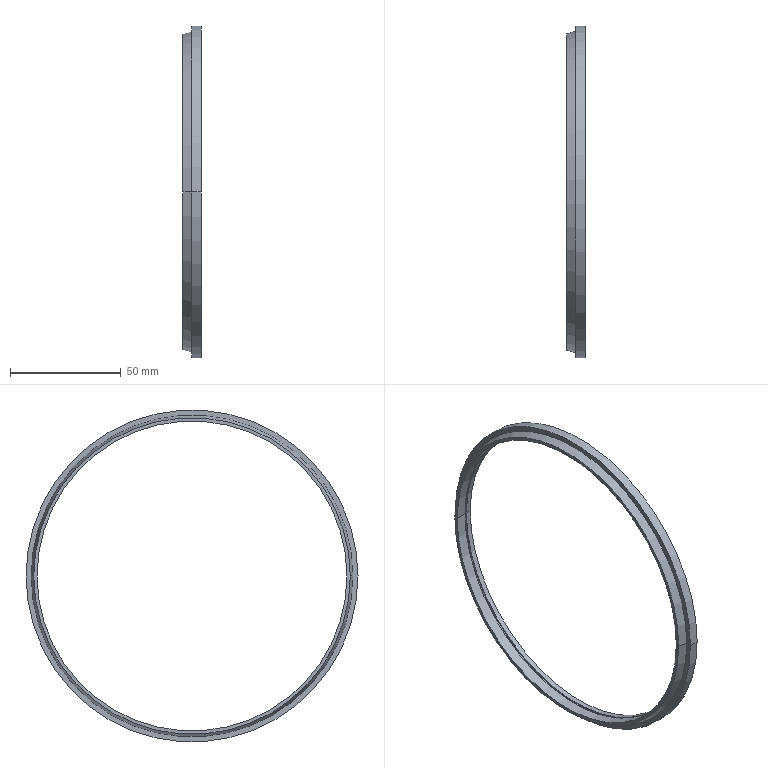Part | SolidWorks | features Revolution 1 | 1 solid | 14 faces | box 8.3 x 150 x 150 mm | volume 13389 mm3 | cylinder 6 | cone 4 | plane 4 | commonest cylinder face diameters 140 x4 150 x2
STEP:
#1=CARTESIAN_POINT('',(-70.,71.5,0.));
#2=VERTEX_POINT('',#1);
#3=CARTESIAN_POINT('',(-70.,-71.5,0.));
#4=VERTEX_POINT('',#3);
#5=CARTESIAN_POINT('',(-70.,0.,0.));
#6=DIRECTION('',(1.,0.,0.));
#7=DIRECTION('',(0.,1.,0.));
#8=AXIS2_PLACEMENT_3D('',#5,#6,#7);
#9=CIRCLE('',#8,71.5);
#10=EDGE_CURVE('',#2,#4,#9,.T.);
#11=ORIENTED_EDGE('',*,*,#10,.T.);
#12=CARTESIAN_POINT('',(-66.,-72.65,0.));
#13=VERTEX_POINT('',#12);
#14=CARTESIAN_POINT('',(-66.,-72.65,0.));
#15=DIRECTION('',(0.9611,-0.2763,0.));
#16=VECTOR('',#15,1000.);
#17=LINE('',#14,#16);
#18=EDGE_CURVE('',#4,#13,#17,.T.);
#19=ORIENTED_EDGE('',*,*,#18,.T.);
#20=CARTESIAN_POINT('',(-66.,72.65,0.));
#21=VERTEX_POINT('',#20);
#22=CARTESIAN_POINT('',(-66.,0.,0.));
#23=DIRECTION('',(1.,0.,0.));
#24=DIRECTION('',(0.,1.,0.));
#25=AXIS2_PLACEMENT_3D('',#22,#23,#24);
#26=CIRCLE('',#25,72.65);
#27=EDGE_CURVE('',#21,#13,#26,.T.);
#28=ORIENTED_EDGE('',*,*,#27,.F.);
#29=CARTESIAN_POINT('',(-66.,72.65,0.));
#30=DIRECTION('',(0.9611,0.2763,0.));
#31=VECTOR('',#30,1000.);
#32=LINE('',#29,#31);
#33=EDGE_CURVE('',#2,#21,#32,.T.);
#34=ORIENTED_EDGE('',*,*,#33,.F.);
#35=EDGE_LOOP('',(#11,#19,#28,#34));
#36=FACE_OUTER_BOUND('',#35,.T.);
#37=CARTESIAN_POINT('',(-66.,0.,0.));
#38=DIRECTION('',(1.,0.,0.));
#39=DIRECTION('',(0.,1.,0.));
#40=AXIS2_PLACEMENT_3D('',#37,#38,#39);
#41=CONICAL_SURFACE('',#40,72.65,0.2799);
#42=ADVANCED_FACE('',(#36),#41,.T.);
#43=CARTESIAN_POINT('',(-70.,-70.,0.));
#44=VERTEX_POINT('',#43);
#45=CARTESIAN_POINT('',(-70.,70.,0.));
#46=VERTEX_POINT('',#45);
#47=CARTESIAN_POINT('',(-70.,0.,0.));
#48=DIRECTION('',(1.,0.,0.));
#49=DIRECTION('',(0.,1.,0.));
#50=AXIS2_PLACEMENT_3D('',#47,#48,#49);
#51=CIRCLE('',#50,70.);
#52=EDGE_CURVE('',#44,#46,#51,.T.);
#53=ORIENTED_EDGE('',*,*,#52,.F.);
#54=CARTESIAN_POINT('',(-65.05,-70.,0.));
#55=VERTEX_POINT('',#54);
#56=CARTESIAN_POINT('',(0.,-70.,0.));
#57=DIRECTION('',(1.,0.,0.));
#58=VECTOR('',#57,1000.);
#59=LINE('',#56,#58);
#60=EDGE_CURVE('',#44,#55,#59,.T.);
#61=ORIENTED_EDGE('',*,*,#60,.T.);
#62=CARTESIAN_POINT('',(-65.05,70.,0.));
#63=VERTEX_POINT('',#62);
#64=CARTESIAN_POINT('',(-65.05,0.,0.));
#65=DIRECTION('',(1.,0.,0.));
#66=DIRECTION('',(0.,1.,0.));
#67=AXIS2_PLACEMENT_3D('',#64,#65,#66);
#68=CIRCLE('',#67,70.);
#69=EDGE_CURVE('',#55,#63,#68,.T.);
#70=ORIENTED_EDGE('',*,*,#69,.T.);
#71=CARTESIAN_POINT('',(0.,70.,0.));
#72=DIRECTION('',(1.,0.,0.));
#73=VECTOR('',#72,1000.);
#74=LINE('',#71,#73);
#75=EDGE_CURVE('',#46,#63,#74,.T.);
#76=ORIENTED_EDGE('',*,*,#75,.F.);
#77=EDGE_LOOP('',(#53,#61,#70,#76));
#78=FACE_OUTER_BOUND('',#77,.T.);
#79=CARTESIAN_POINT('',(0.,0.,0.));
#80=DIRECTION('',(1.,0.,0.));
#81=DIRECTION('',(0.,1.,0.));
#82=AXIS2_PLACEMENT_3D('',#79,#80,#81);
#83=CYLINDRICAL_SURFACE('',#82,70.);
#84=ADVANCED_FACE('',(#78),#83,.F.);
#85=ORIENTED_EDGE('',*,*,#69,.F.);
#86=CARTESIAN_POINT('',(-64.128,-70.547,0.));
#87=VERTEX_POINT('',#86);
#88=CARTESIAN_POINT('',(-65.05,-70.,0.));
#89=DIRECTION('',(0.8601,-0.5101,0.));
#90=VECTOR('',#89,1000.);
#91=LINE('',#88,#90);
#92=EDGE_CURVE('',#55,#87,#91,.T.);
#93=ORIENTED_EDGE('',*,*,#92,.T.);
#94=CARTESIAN_POINT('',(-64.128,70.547,0.));
#95=VERTEX_POINT('',#94);
#96=CARTESIAN_POINT('',(-64.128,0.,0.));
#97=DIRECTION('',(1.,0.,0.));
#98=DIRECTION('',(0.,1.,0.));
#99=AXIS2_PLACEMENT_3D('',#96,#97,#98);
#100=CIRCLE('',#99,70.547);
#101=EDGE_CURVE('',#87,#95,#100,.T.);
#102=ORIENTED_EDGE('',*,*,#101,.T.);
#103=CARTESIAN_POINT('',(-65.05,70.,0.));
#104=DIRECTION('',(0.8601,0.5101,0.));
#105=VECTOR('',#104,1000.);
#106=LINE('',#103,#105);
#107=EDGE_CURVE('',#63,#95,#106,.T.);
#108=ORIENTED_EDGE('',*,*,#107,.F.);
#109=EDGE_LOOP('',(#85,#93,#102,#108));
#110=FACE_OUTER_BOUND('',#109,.T.);
#111=CARTESIAN_POINT('',(-65.05,0.,0.));
#112=DIRECTION('',(1.,0.,0.));
#113=DIRECTION('',(0.,1.,0.));
#114=AXIS2_PLACEMENT_3D('',#111,#112,#113);
#115=CONICAL_SURFACE('',#114,70.,0.5353);
#116=ADVANCED_FACE('',(#110),#115,.F.);
#117=CARTESIAN_POINT('',(-64.128,-70.,0.));
#118=VERTEX_POINT('',#117);
#119=CARTESIAN_POINT('',(-64.128,70.,0.));
#120=VERTEX_POINT('',#119);
#121=CARTESIAN_POINT('',(-64.128,0.,0.));
#122=DIRECTION('',(1.,0.,0.));
#123=DIRECTION('',(0.,1.,0.));
#124=AXIS2_PLACEMENT_3D('',#121,#122,#123);
#125=CIRCLE('',#124,70.);
#126=EDGE_CURVE('',#118,#120,#125,.T.);
#127=ORIENTED_EDGE('',*,*,#126,.F.);
#128=CARTESIAN_POINT('',(-61.7,-70.,0.));
#129=VERTEX_POINT('',#128);
#130=CARTESIAN_POINT('',(0.,-70.,0.));
#131=DIRECTION('',(1.,0.,0.));
#132=VECTOR('',#131,1000.);
#133=LINE('',#130,#132);
#134=EDGE_CURVE('',#118,#129,#133,.T.);
#135=ORIENTED_EDGE('',*,*,#134,.T.);
#136=CARTESIAN_POINT('',(-61.7,70.,0.));
#137=VERTEX_POINT('',#136);
#138=CARTESIAN_POINT('',(-61.7,0.,0.));
#139=DIRECTION('',(1.,0.,0.));
#140=DIRECTION('',(0.,1.,0.));
#141=AXIS2_PLACEMENT_3D('',#138,#139,#140);
#142=CIRCLE('',#141,70.);
#143=EDGE_CURVE('',#129,#137,#142,.T.);
#144=ORIENTED_EDGE('',*,*,#143,.T.);
#145=CARTESIAN_POINT('',(0.,70.,0.));
#146=DIRECTION('',(1.,0.,0.));
#147=VECTOR('',#146,1000.);
#148=LINE('',#145,#147);
#149=EDGE_CURVE('',#120,#137,#148,.T.);
#150=ORIENTED_EDGE('',*,*,#149,.F.);
#151=EDGE_LOOP('',(#127,#135,#144,#150));
#152=FACE_OUTER_BOUND('',#151,.T.);
#153=CARTESIAN_POINT('',(0.,0.,0.));
#154=DIRECTION('',(1.,0.,0.));
#155=DIRECTION('',(0.,1.,0.));
#156=AXIS2_PLACEMENT_3D('',#153,#154,#155);
#157=CYLINDRICAL_SURFACE('',#156,70.);
#158=ADVANCED_FACE('',(#152),#157,.F.);
#159=CARTESIAN_POINT('',(-66.,75.,0.));
#160=VERTEX_POINT('',#159);
#161=CARTESIAN_POINT('',(-66.,-75.,0.));
#162=VERTEX_POINT('',#161);
#163=CARTESIAN_POINT('',(-66.,0.,0.));
#164=DIRECTION('',(1.,0.,0.));
#165=DIRECTION('',(0.,1.,0.));
#166=AXIS2_PLACEMENT_3D('',#163,#164,#165);
#167=CIRCLE('',#166,75.);
#168=EDGE_CURVE('',#160,#162,#167,.T.);
#169=ORIENTED_EDGE('',*,*,#168,.T.);
#170=CARTESIAN_POINT('',(-61.7,-75.,0.));
#171=VERTEX_POINT('',#170);
#172=CARTESIAN_POINT('',(0.,-75.,0.));
#173=DIRECTION('',(1.,0.,0.));
#174=VECTOR('',#173,1000.);
#175=LINE('',#172,#174);
#176=EDGE_CURVE('',#162,#171,#175,.T.);
#177=ORIENTED_EDGE('',*,*,#176,.T.);
#178=CARTESIAN_POINT('',(-61.7,75.,0.));
#179=VERTEX_POINT('',#178);
#180=CARTESIAN_POINT('',(-61.7,0.,0.));
#181=DIRECTION('',(1.,0.,0.));
#182=DIRECTION('',(0.,1.,0.));
#183=AXIS2_PLACEMENT_3D('',#180,#181,#182);
#184=CIRCLE('',#183,75.);
#185=EDGE_CURVE('',#179,#171,#184,.T.);
#186=ORIENTED_EDGE('',*,*,#185,.F.);
#187=CARTESIAN_POINT('',(0.,75.,0.));
#188=DIRECTION('',(1.,0.,0.));
#189=VECTOR('',#188,1000.);
#190=LINE('',#187,#189);
#191=EDGE_CURVE('',#160,#179,#190,.T.);
#192=ORIENTED_EDGE('',*,*,#191,.F.);
#193=EDGE_LOOP('',(#169,#177,#186,#192));
#194=FACE_OUTER_BOUND('',#193,.T.);
#195=CARTESIAN_POINT('',(0.,0.,0.));
#196=DIRECTION('',(1.,0.,0.));
#197=DIRECTION('',(0.,1.,0.));
#198=AXIS2_PLACEMENT_3D('',#195,#196,#197);
#199=CYLINDRICAL_SURFACE('',#198,75.);
#200=ADVANCED_FACE('',(#194),#199,.T.);
#201=ORIENTED_EDGE('',*,*,#176,.F.);
#202=CARTESIAN_POINT('',(-66.,0.,0.));
#203=DIRECTION('',(1.,0.,0.));
#204=DIRECTION('',(0.,1.,0.));
#205=AXIS2_PLACEMENT_3D('',#202,#203,#204);
#206=CIRCLE('',#205,75.);
#207=EDGE_CURVE('',#162,#160,#206,.T.);
#208=ORIENTED_EDGE('',*,*,#207,.T.);
#209=ORIENTED_EDGE('',*,*,#191,.T.);
#210=CARTESIAN_POINT('',(-61.7,0.,0.));
#211=DIRECTION('',(1.,0.,0.));
#212=DIRECTION('',(0.,1.,0.));
#213=AXIS2_PLACEMENT_3D('',#210,#211,#212);
#214=CIRCLE('',#213,75.);
#215=EDGE_CURVE('',#171,#179,#214,.T.);
#216=ORIENTED_EDGE('',*,*,#215,.F.);
#217=EDGE_LOOP('',(#201,#208,#209,#216));
#218=FACE_OUTER_BOUND('',#217,.T.);
#219=CARTESIAN_POINT('',(0.,0.,0.));
#220=DIRECTION('',(1.,0.,0.));
#221=DIRECTION('',(0.,1.,0.));
#222=AXIS2_PLACEMENT_3D('',#219,#220,#221);
#223=CYLINDRICAL_SURFACE('',#222,75.);
#224=ADVANCED_FACE('',(#218),#223,.T.);
#225=CARTESIAN_POINT('',(-61.7,0.,0.));
#226=DIRECTION('',(1.,0.,0.));
#227=DIRECTION('',(0.,1.,0.));
#228=AXIS2_PLACEMENT_3D('',#225,#226,#227);
#229=CIRCLE('',#228,70.);
#230=EDGE_CURVE('',#137,#129,#229,.T.);
#231=ORIENTED_EDGE('',*,*,#230,.F.);
#232=ORIENTED_EDGE('',*,*,#143,.F.);
#233=EDGE_LOOP('',(#231,#232));
#234=FACE_BOUND('',#233,.T.);
#235=ORIENTED_EDGE('',*,*,#185,.T.);
#236=ORIENTED_EDGE('',*,*,#215,.T.);
#237=EDGE_LOOP('',(#235,#236));
#238=FACE_OUTER_BOUND('',#237,.T.);
#239=CARTESIAN_POINT('',(-61.7,75.,0.));
#240=DIRECTION('',(-1.,0.,0.));
#241=DIRECTION('',(0.,-1.,0.));
#242=AXIS2_PLACEMENT_3D('',#239,#240,#241);
#243=PLANE('',#242);
#244=ADVANCED_FACE('',(#234,#238),#243,.F.);
#245=ORIENTED_EDGE('',*,*,#134,.F.);
#246=CARTESIAN_POINT('',(-64.128,0.,0.));
#247=DIRECTION('',(1.,0.,0.));
#248=DIRECTION('',(0.,1.,0.));
#249=AXIS2_PLACEMENT_3D('',#246,#247,#248);
#250=CIRCLE('',#249,70.);
#251=EDGE_CURVE('',#120,#118,#250,.T.);
#252=ORIENTED_EDGE('',*,*,#251,.F.);
#253=ORIENTED_EDGE('',*,*,#149,.T.);
#254=ORIENTED_EDGE('',*,*,#230,.T.);
#255=EDGE_LOOP('',(#245,#252,#253,#254));
#256=FACE_OUTER_BOUND('',#255,.T.);
#257=CARTESIAN_POINT('',(0.,0.,0.));
#258=DIRECTION('',(1.,0.,0.));
#259=DIRECTION('',(0.,1.,0.));
#260=AXIS2_PLACEMENT_3D('',#257,#258,#259);
#261=CYLINDRICAL_SURFACE('',#260,70.);
#262=ADVANCED_FACE('',(#256),#261,.F.);
#263=ORIENTED_EDGE('',*,*,#251,.T.);
#264=ORIENTED_EDGE('',*,*,#126,.T.);
#265=EDGE_LOOP('',(#263,#264));
#266=FACE_BOUND('',#265,.T.);
#267=CARTESIAN_POINT('',(-64.128,0.,0.));
#268=DIRECTION('',(1.,0.,0.));
#269=DIRECTION('',(0.,1.,0.));
#270=AXIS2_PLACEMENT_3D('',#267,#268,#269);
#271=CIRCLE('',#270,70.547);
#272=EDGE_CURVE('',#95,#87,#271,.T.);
#273=ORIENTED_EDGE('',*,*,#272,.F.);
#274=ORIENTED_EDGE('',*,*,#101,.F.);
#275=EDGE_LOOP('',(#273,#274));
#276=FACE_OUTER_BOUND('',#275,.T.);
#277=CARTESIAN_POINT('',(-64.128,70.547,0.));
#278=DIRECTION('',(-1.,0.,0.));
#279=DIRECTION('',(0.,-1.,0.));
#280=AXIS2_PLACEMENT_3D('',#277,#278,#279);
#281=PLANE('',#280);
#282=ADVANCED_FACE('',(#266,#276),#281,.T.);
#283=ORIENTED_EDGE('',*,*,#92,.F.);
#284=CARTESIAN_POINT('',(-65.05,0.,0.));
#285=DIRECTION('',(1.,0.,0.));
#286=DIRECTION('',(0.,1.,0.));
#287=AXIS2_PLACEMENT_3D('',#284,#285,#286);
#288=CIRCLE('',#287,70.);
#289=EDGE_CURVE('',#63,#55,#288,.T.);
#290=ORIENTED_EDGE('',*,*,#289,.F.);
#291=ORIENTED_EDGE('',*,*,#107,.T.);
#292=ORIENTED_EDGE('',*,*,#272,.T.);
#293=EDGE_LOOP('',(#283,#290,#291,#292));
#294=FACE_OUTER_BOUND('',#293,.T.);
#295=CARTESIAN_POINT('',(-65.05,0.,0.));
#296=DIRECTION('',(1.,0.,0.));
#297=DIRECTION('',(0.,1.,0.));
#298=AXIS2_PLACEMENT_3D('',#295,#296,#297);
#299=CONICAL_SURFACE('',#298,70.,0.5353);
#300=ADVANCED_FACE('',(#294),#299,.F.);
#301=ORIENTED_EDGE('',*,*,#60,.F.);
#302=CARTESIAN_POINT('',(-70.,0.,0.));
#303=DIRECTION('',(1.,0.,0.));
#304=DIRECTION('',(0.,1.,0.));
#305=AXIS2_PLACEMENT_3D('',#302,#303,#304);
#306=CIRCLE('',#305,70.);
#307=EDGE_CURVE('',#46,#44,#306,.T.);
#308=ORIENTED_EDGE('',*,*,#307,.F.);
#309=ORIENTED_EDGE('',*,*,#75,.T.);
#310=ORIENTED_EDGE('',*,*,#289,.T.);
#311=EDGE_LOOP('',(#301,#308,#309,#310));
#312=FACE_OUTER_BOUND('',#311,.T.);
#313=CARTESIAN_POINT('',(0.,0.,0.));
#314=DIRECTION('',(1.,0.,0.));
#315=DIRECTION('',(0.,1.,0.));
#316=AXIS2_PLACEMENT_3D('',#313,#314,#315);
#317=CYLINDRICAL_SURFACE('',#316,70.);
#318=ADVANCED_FACE('',(#312),#317,.F.);
#319=ORIENTED_EDGE('',*,*,#10,.F.);
#320=CARTESIAN_POINT('',(-70.,0.,0.));
#321=DIRECTION('',(1.,0.,0.));
#322=DIRECTION('',(0.,1.,0.));
#323=AXIS2_PLACEMENT_3D('',#320,#321,#322);
#324=CIRCLE('',#323,71.5);
#325=EDGE_CURVE('',#4,#2,#324,.T.);
#326=ORIENTED_EDGE('',*,*,#325,.F.);
#327=EDGE_LOOP('',(#319,#326));
#328=FACE_OUTER_BOUND('',#327,.T.);
#329=ORIENTED_EDGE('',*,*,#307,.T.);
#330=ORIENTED_EDGE('',*,*,#52,.T.);
#331=EDGE_LOOP('',(#329,#330));
#332=FACE_BOUND('',#331,.T.);
#333=CARTESIAN_POINT('',(-70.,70.,0.));
#334=DIRECTION('',(1.,0.,0.));
#335=DIRECTION('',(0.,1.,0.));
#336=AXIS2_PLACEMENT_3D('',#333,#334,#335);
#337=PLANE('',#336);
#338=ADVANCED_FACE('',(#328,#332),#337,.F.);
#339=ORIENTED_EDGE('',*,*,#18,.F.);
#340=ORIENTED_EDGE('',*,*,#325,.T.);
#341=ORIENTED_EDGE('',*,*,#33,.T.);
#342=CARTESIAN_POINT('',(-66.,0.,0.));
#343=DIRECTION('',(1.,0.,0.));
#344=DIRECTION('',(0.,1.,0.));
#345=AXIS2_PLACEMENT_3D('',#342,#343,#344);
#346=CIRCLE('',#345,72.65);
#347=EDGE_CURVE('',#13,#21,#346,.T.);
#348=ORIENTED_EDGE('',*,*,#347,.F.);
#349=EDGE_LOOP('',(#339,#340,#341,#348));
#350=FACE_OUTER_BOUND('',#349,.T.);
#351=CARTESIAN_POINT('',(-66.,0.,0.));
#352=DIRECTION('',(1.,0.,0.));
#353=DIRECTION('',(0.,1.,0.));
#354=AXIS2_PLACEMENT_3D('',#351,#352,#353);
#355=CONICAL_SURFACE('',#354,72.65,0.2799);
#356=ADVANCED_FACE('',(#350),#355,.T.);
#357=ORIENTED_EDGE('',*,*,#27,.T.);
#358=ORIENTED_EDGE('',*,*,#347,.T.);
#359=EDGE_LOOP('',(#357,#358));
#360=FACE_BOUND('',#359,.T.);
#361=ORIENTED_EDGE('',*,*,#168,.F.);
#362=ORIENTED_EDGE('',*,*,#207,.F.);
#363=EDGE_LOOP('',(#361,#362));
#364=FACE_OUTER_BOUND('',#363,.T.);
#365=CARTESIAN_POINT('',(-66.,75.,0.));
#366=DIRECTION('',(-1.,0.,0.));
#367=DIRECTION('',(0.,-1.,0.));
#368=AXIS2_PLACEMENT_3D('',#365,#366,#367);
#369=PLANE('',#368);
#370=ADVANCED_FACE('',(#360,#364),#369,.T.);
#371=CLOSED_SHELL('',(#42,#84,#116,#158,#200,#224,#244,#262,#282,#300,#318,#338,#356,#370));
#372=MANIFOLD_SOLID_BREP('',#371);
#373=CARTESIAN_POINT('',(0.,0.,0.));
#374=DIRECTION('',(0.,0.,1.));
#375=DIRECTION('',(1.,0.,0.));
#376=AXIS2_PLACEMENT_3D('',#373,#374,#375);
#377=(LENGTH_UNIT()NAMED_UNIT(*)SI_UNIT(.MILLI.,.METRE.));
#378=UNCERTAINTY_MEASURE_WITH_UNIT(LENGTH_MEASURE(0.00001),#377,'','');
#379=(NAMED_UNIT(*)PLANE_ANGLE_UNIT()SI_UNIT($,.RADIAN.));
#380=(NAMED_UNIT(*)SI_UNIT($,.STERADIAN.)SOLID_ANGLE_UNIT());
#381=(GEOMETRIC_REPRESENTATION_CONTEXT(3)GLOBAL_UNCERTAINTY_ASSIGNED_CONTEXT((#378))GLOBAL_UNIT_ASSIGNED_CONTEXT((#377,#379,#380))REPRESENTATION_CONTEXT('',''));
#382=ADVANCED_BREP_SHAPE_REPRESENTATION('',(#372,#376),#381);